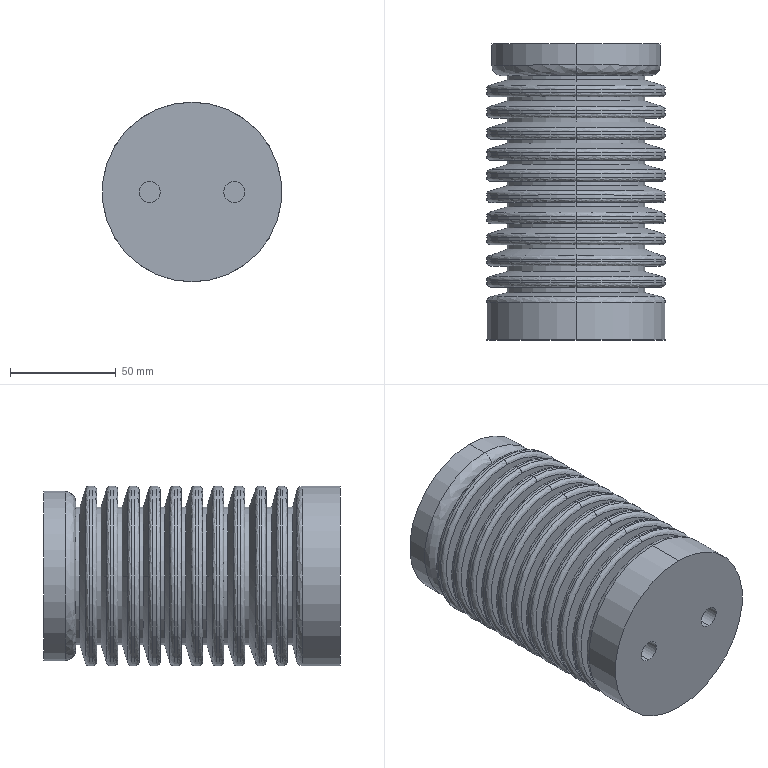Part | SolidWorks | features BaseBody 1 | 1 solid | 137 faces | box 85 x 140 x 85 mm | volume 678423 mm3 | cylinder 54 | spline 44 | cone 22 | plane 17 | commonest cylinder face diameters 65 x22 85 x22 10 x8 80 x2